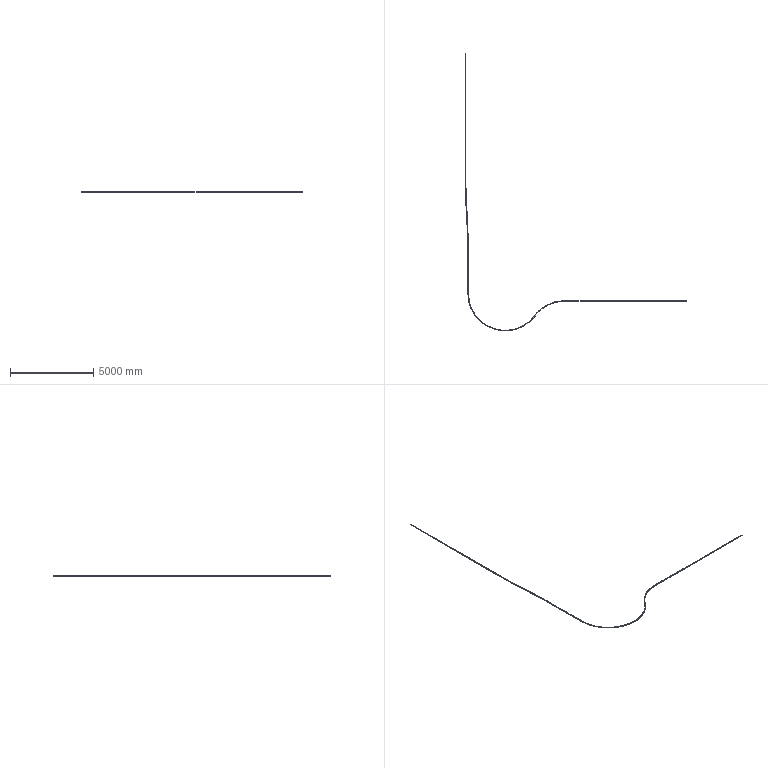Part | SolidWorks | features Sweep 1 | 1 solid | 22 faces | box 13271 x 16645 x 30 mm | volume 5014402 mm3 | spline 14 | plane 8